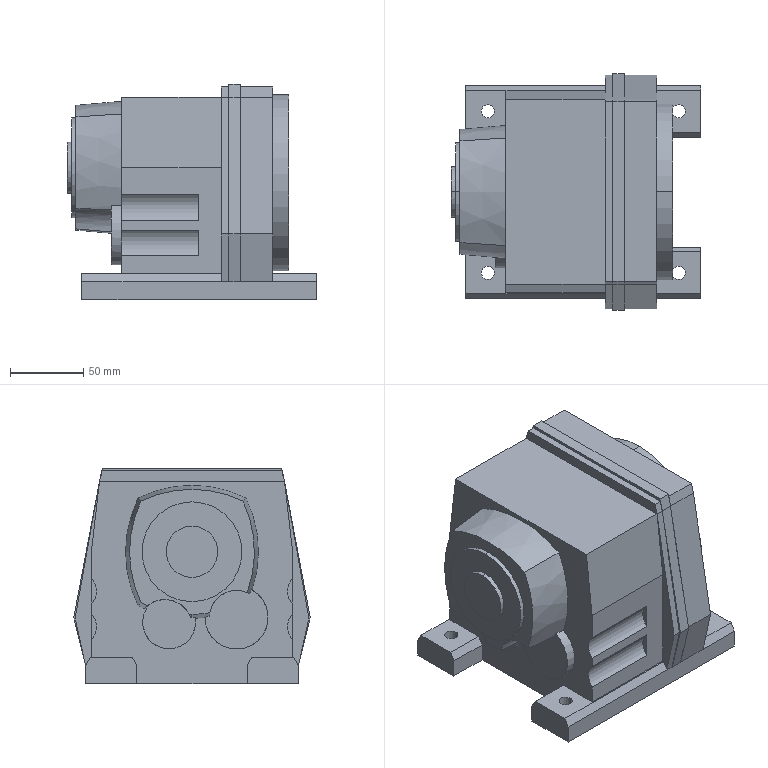Part | SolidWorks | features BaseBody 1 | 1 solid | 117 faces | box 170 x 161 x 147 mm | volume 2353426 mm3 | plane 77 | cylinder 34 | cone 6 | commonest cylinder face diameters 6 x8 9 x8 24 x4 35 x2 36 x2 43 x2